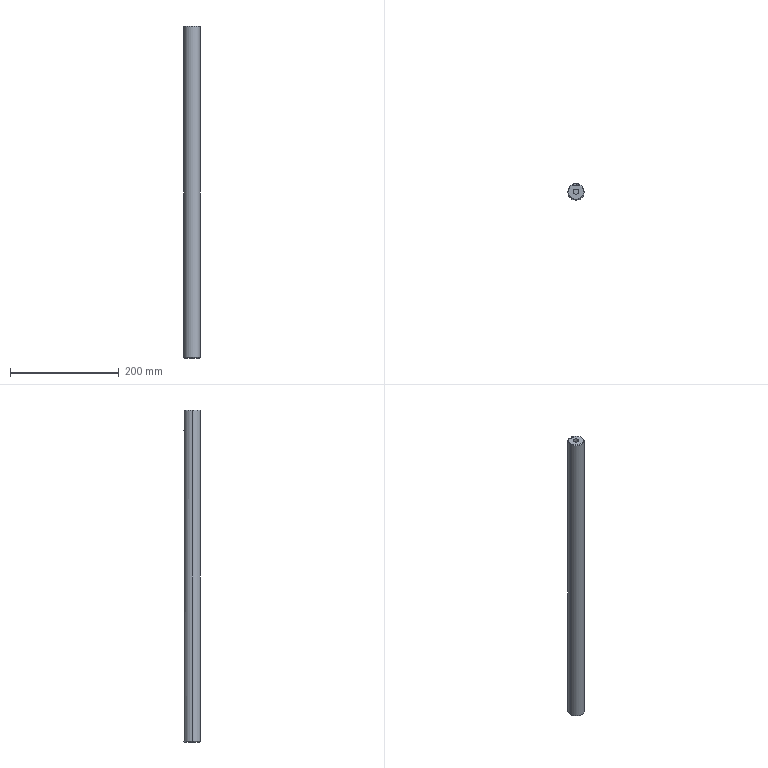Part | STEP file | Shaft dia 25 for feeder1V11 | 1 solid | 20 faces | box 30 x 30 x 609.6 mm | volume 424964 mm3 | cylinder 8 | plane 7 | cone 5 | commonest cylinder face diameters 10 x4 8 x2 30 x2